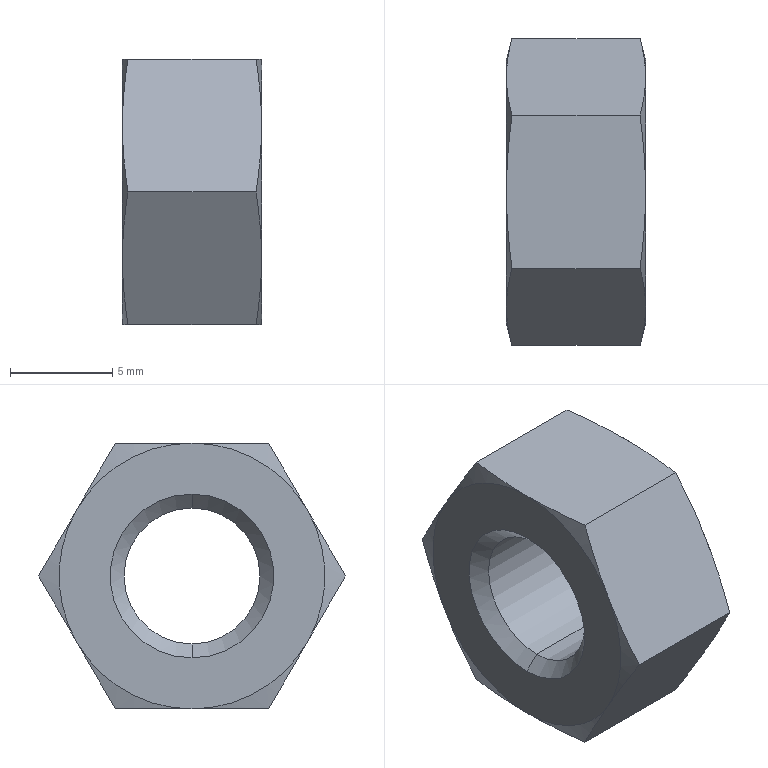Part | STEP file | 0217_Z_SBSP8-30-2 | 1 solid | 26 faces | box 6.8 x 15.011 x 13 mm | volume 746.792 mm3 | cone 16 | plane 8 | cylinder 2 | commonest cylinder face diameters 6.647 x2